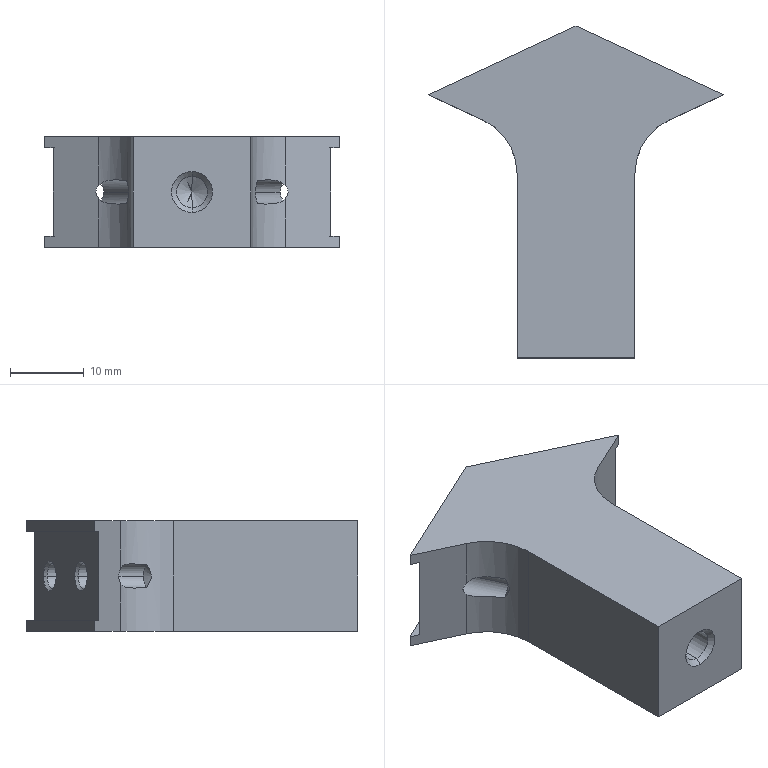Part | STEP file | B1-013 | 1 solid | 49 faces | box 40 x 45 x 15 mm | volume 11495 mm3 | cone 22 | plane 15 | cylinder 12 | commonest cylinder face diameters 3.3 x8 4.2 x2 16 x2